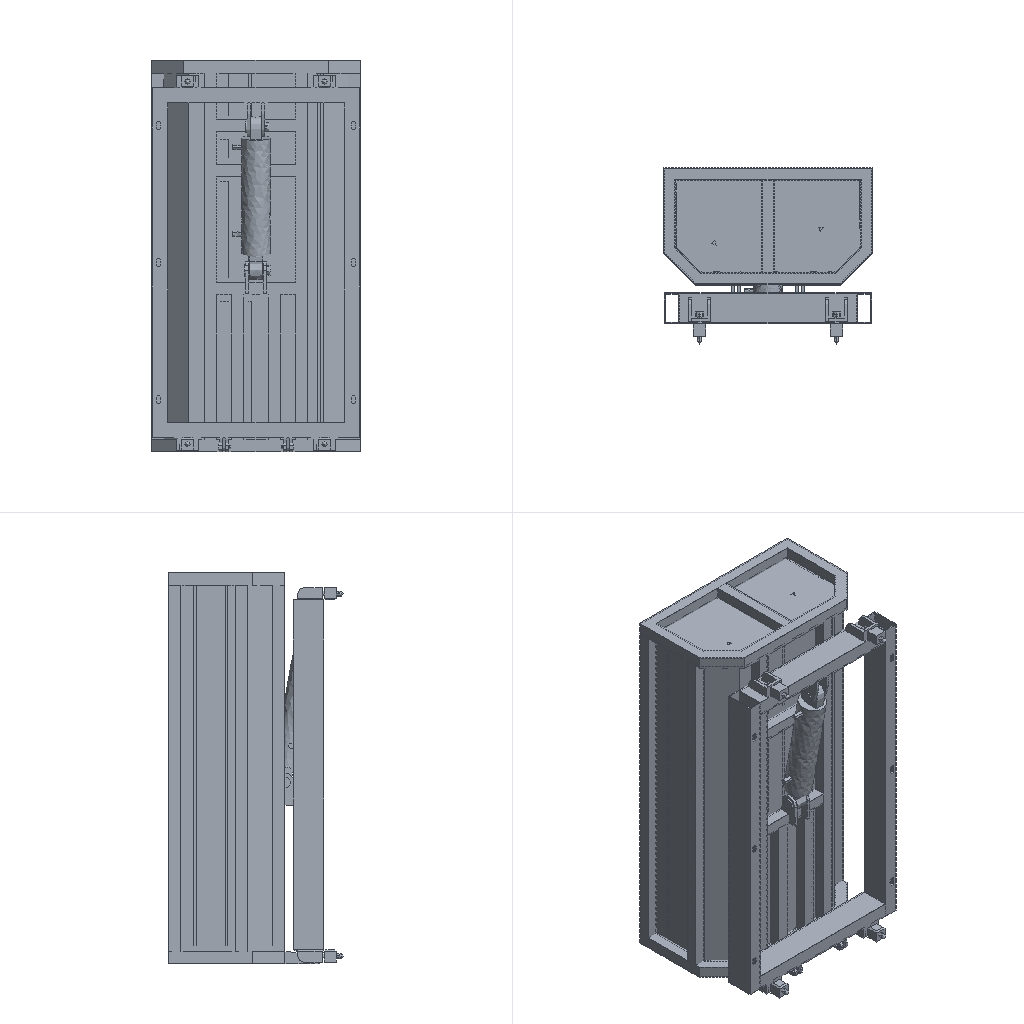Simulation study | ansys workbench
Ansys APDL input file, long lists of numbers shortened:
/batch
/config,noeldb,1     ! force off writing results to database
*get,_wallstrt,active,,time,wall
! ANSYS input file written by Workbench version 2022 R1
! File used for geometry attach:
/title,wbnew--____ (A5)
! ****** Begin Custom Load Command Snippet ******
/COM, ACT Extensions:
/COM,     LSDYNA, 2021.1
/COM,
! ****** End   Custom Load Command Snippet ******
*DIM,_wb_ProjectScratch_dir,string,248
_wb_ProjectScratch_dir(1) = ''
*DIM,_wb_SolverFiles_dir,string,248
_wb_SolverFiles_dir(1) = ''
*DIM,_wb_userfiles_dir,string,248
_wb_userfiles_dir(1) = ''
/com,--- Data in consistent MKS units. See Solving Units in the help system for more information.
/units,MKS
/nopr
/wb,file,start              !  signify a WB generated input file
/prep7
! Turn off shape checking because checks already performed inside WB mesher.
! See help system for more information.
SHPP,OFF,,NOWARN
/nolist
etcon,set             ! allow ANSYS to choose best KEYOP's for 180x elements, resets any applicable keyopt to MAPDL defaults
/com,*********** Nodes for the whole assembly ***********
nblock,3,,236970
(1i9,3e20.9e3)
        1    -3.888006712E-01    -1.500000000E-02    -1.150000000E+00
! (215427 more lines like these left out)
-1
/wb,elem,start            !  set before creation of elements
/com,*********** Elements for Body 1 "__\____-____1" ***********
et,1,186
keyo,1,2,1          ! set full integration on SOLID186
eblock,19,solid,,8694
(19i9)
        1        1        1        1        0        0        0        0       20        0     8776    28866    28867    30619    30620    30469    30468    32181    32180
! (17387 more lines like these left out)
-1
/com,*********** Elements for Body 2 "______3c_____3e_\__________________gb_Mt6728-2002 40__3(1)[1]" ***********
et,2,187
eblock,19,solid,,16742
(19i9)
        2        2        2        2        0        0        0        0       10        0    26722    98215   100703   101303   101302   114147   127238   114152   114151
! (33483 more lines like these left out)
-1
/com,*********** Elements for Body 3 "40X3_______3c_____3e_\____4[1]" ***********
et,3,187
eblock,19,solid,,5167
(19i9)
        3        3        3        3        0        0        0        0       10        0     3609    12186    13249    12762    12380    16239    19847    16237    16235
! (10333 more lines like these left out)
-1
/com,*********** Elements for Body 4 "40X3X1420____3c_____3e_\__________________(gb t6728-2002) 40__3(1)" ***********
et,4,186
keyo,4,2,1          ! set full integration on SOLID186
eblock,19,solid,,976
(19i9)
        4        4        4        4        0        0        0        0       20        0    68502   181284   182140   182324   181348   181346   182322   182323   181347
! (1951 more lines like these left out)
-1
/com,*********** Elements for Body 5 "40X3X1420____3c_____3e_\__________________(gb t6728-2002) 40__3(1)" ***********
et,5,186
keyo,5,2,1          ! set full integration on SOLID186
eblock,19,solid,,976
(19i9)
        5        5        5        5        0        0        0        0       20        0    69478   188196   189052   189236   188260   188258   189234   189235   188259
! (1951 more lines like these left out)
-1
! (41 more sections like these left out)
/wb,elem,end               !  done creating elements
/com,*********** Send User Defined Coordinate System(s) ***********
csys,0
toffst,273.15,  ! Temperature offset from absolute zero
/com,*********** Set Reference Temperature ***********
tref,22.
/wb,mat,start              !  starting to send materials
/com,*********** Send Materials ***********
Temperature = 'TEMP' ! Temperature
MP,DENS,1,7850,	! kg m^-3
MP,ALPX,1,1.2e-05,	! C^-1
MP,C,1,434,	! J kg^-1 C^-1
MP,KXX,1,60.5,	! W m^-1 C^-1
MP,RSVX,1,1.7e-07,	! kg m^3 A^-2 s^-3
MP,EX,1,200000000000,	! Pa
MP,NUXY,1,0.3,
MP,MURX,1,10000,
Temperature = 'TEMP' ! Temperature
MP,DENS,2,7850,	! kg m^-3
MP,ALPX,2,1.2e-05,	! C^-1
MP,C,2,434,	! J kg^-1 C^-1
MP,KXX,2,60.5,	! W m^-1 C^-1
MP,RSVX,2,1.7e-07,	! kg m^3 A^-2 s^-3
MP,EX,2,200000000000,	! Pa
MP,NUXY,2,0.3,
MP,MURX,2,10000,
Temperature = 'TEMP' ! Temperature
MP,DENS,3,7850,	! kg m^-3
MP,ALPX,3,1.2e-05,	! C^-1
MP,C,3,434,	! J kg^-1 C^-1
MP,KXX,3,60.5,	! W m^-1 C^-1
MP,RSVX,3,1.7e-07,	! kg m^3 A^-2 s^-3
MP,EX,3,200000000000,	! Pa
MP,NUXY,3,0.3,
MP,MURX,3,10000,
Temperature = 'TEMP' ! Temperature
MP,DENS,4,7850,	! kg m^-3
MP,ALPX,4,1.2e-05,	! C^-1
MP,C,4,434,	! J kg^-1 C^-1
MP,KXX,4,60.5,	! W m^-1 C^-1
MP,RSVX,4,1.7e-07,	! kg m^3 A^-2 s^-3
MP,EX,4,200000000000,	! Pa
MP,NUXY,4,0.3,
MP,MURX,4,10000,
Temperature = 'TEMP' ! Temperature
MP,DENS,5,7850,	! kg m^-3
MP,ALPX,5,1.2e-05,	! C^-1
MP,C,5,434,	! J kg^-1 C^-1
MP,KXX,5,60.5,	! W m^-1 C^-1
MP,RSVX,5,1.7e-07,	! kg m^3 A^-2 s^-3
MP,EX,5,200000000000,	! Pa
MP,NUXY,5,0.3,
MP,MURX,5,10000,
Temperature = 'TEMP' ! Temperature
MP,DENS,6,7850,	! kg m^-3
MP,ALPX,6,1.2e-05,	! C^-1
MP,C,6,434,	! J kg^-1 C^-1
MP,KXX,6,60.5,	! W m^-1 C^-1
MP,RSVX,6,1.7e-07,	! kg m^3 A^-2 s^-3
MP,EX,6,200000000000,	! Pa
MP,NUXY,6,0.3,
MP,MURX,6,10000,
Temperature = 'TEMP' ! Temperature
MP,DENS,7,7850,	! kg m^-3
MP,ALPX,7,1.2e-05,	! C^-1
MP,C,7,434,	! J kg^-1 C^-1
MP,KXX,7,60.5,	! W m^-1 C^-1
MP,RSVX,7,1.7e-07,	! kg m^3 A^-2 s^-3
MP,EX,7,200000000000,	! Pa
MP,NUXY,7,0.3,
MP,MURX,7,10000,
Temperature = 'TEMP' ! Temperature
MP,DENS,8,7850,	! kg m^-3
MP,ALPX,8,1.2e-05,	! C^-1
MP,C,8,434,	! J kg^-1 C^-1
MP,KXX,8,60.5,	! W m^-1 C^-1
MP,RSVX,8,1.7e-07,	! kg m^3 A^-2 s^-3
MP,EX,8,200000000000,	! Pa
MP,NUXY,8,0.3,
MP,MURX,8,10000,
Temperature = 'TEMP' ! Temperature
MP,DENS,9,7850,	! kg m^-3
MP,ALPX,9,1.2e-05,	! C^-1
MP,C,9,434,	! J kg^-1 C^-1
MP,KXX,9,60.5,	! W m^-1 C^-1
MP,RSVX,9,1.7e-07,	! kg m^3 A^-2 s^-3
MP,EX,9,200000000000,	! Pa
! (335 more lines like these left out)
/wb,mat,end                !  done sending materials
!************************* Model Summary ********************
!__\____-____1,	结构钢,	matid,	1
!______3c_____3e_\__________________gb_Mt6728-2002 40__3(1)[1],	结构钢,	matid,	2
!40X3_______3c_____3e_\____4[1],	结构钢,	matid,	3
! (45 more lines like these left out)
*get,_xmin,node,,mnloc,x
*get,_ymin,node,,mnloc,y
*get,_zmin,node,,mnloc,z
*get,_xmax,node,,mxloc,x
*get,_ymax,node,,mxloc,y
*get,_zmax,node,,mxloc,z
_ASMDIAG=(_xmax-_xmin)*(_xmax-_xmin)+(_ymax-_ymin)*(_ymax-_ymin)+(_zmax-_zmin)*(_zmax-_zmin)
_ASMDIAG=SQRT(_ASMDIAG)
/wb,contact,start          !  starting to send contact
/com,*********** Create Contact "接触区域" ***********
/com,            Real Constant Set For Above Contact Is 48 & 47
*set,tid,48
*set,cid,47
r,tid
r,cid
et,tid,170
et,cid,174
eblock,10,,,1504
(15i9)
   142848       48       48       48        0    25380    25381    25319    25318    47320    47139    47134    47135
! (1503 more lines like these left out)
-1
eblock,10,,,1504
(15i9)
   144352       47       47       47        0    25380    25381    25319    25318    47320    47139    47134    47135
! (1503 more lines like these left out)
-1
eblock,10,,,1368
(15i9)
   145856       47       48       47        0    97493   100730    99290    99290   108211   120892    99290   108208
! (1367 more lines like these left out)
-1
eblock,10,,,1368
(15i9)
   147224       48       47       48        0    97493   100730    99290    99290   108211   120892    99290   108208
! (1367 more lines like these left out)
-1
keyo,cid,8,2               ! auto create asymmetric contact (from Program Controlled setting)
keyo,cid,10,0              ! adjust contact stiffness each NR iteration (from Program Controlled setting)
keyo,cid,12,5              ! bonded always
keyo,cid,2,2               ! MPC contact.  Valid only for bonded or no separation.  Requires nodal detection
keyo,cid,4,2               ! on nodal point - normal to target surface (from Program Controlled setting)
keyo,cid,9,1               ! ignore initial gaps/penetration
keyo,cid,7,0               ! No Prediction
rmod,tid,3,10.      ! FKN
rmod,tid,5,0.       ! ICONT
rmod,tid,6,0.       ! PINB
rmod,tid,10,0.      ! CNOF
rmod,tid,12,0.      ! FKT
rmod,tid,36,161     ! WB DSID
rmod,cid,3,10.      ! FKN
rmod,cid,5,0.       ! ICONT
rmod,cid,6,0.       ! PINB
rmod,cid,10,0.      ! CNOF
rmod,cid,12,0.      ! FKT
rmod,cid,36,161     ! WB DSID
/com,*********** Create Contact "接触区域 2" ***********
/com,            Real Constant Set For Above Contact Is 50 & 49
*set,tid,50
*set,cid,49
r,tid
r,cid
et,tid,170
et,cid,174
eblock,10,,,378
(15i9)
   148592       50       50       50        0    24286    22612    22550    22549    39058    38934    38931    38932
! (377 more lines like these left out)
-1
eblock,10,,,378
(15i9)
   148970       49       49       49        0    24286    22612    22550    22549    39058    38934    38931    38932
! (377 more lines like these left out)
-1
eblock,10,,,440
(15i9)
   149348       49       50       49        0    12046    12616    13485    13485    15139    19132    13485    15144
! (439 more lines like these left out)
-1
eblock,10,,,440
(15i9)
   149788       50       49       50        0    12046    12616    13485    13485    15139    19132    13485    15144
! (439 more lines like these left out)
-1
keyo,cid,8,2               ! auto create asymmetric contact (from Program Controlled setting)
keyo,cid,10,0              ! adjust contact stiffness each NR iteration (from Program Controlled setting)
keyo,cid,12,5              ! bonded always
keyo,cid,2,2               ! MPC contact.  Valid only for bonded or no separation.  Requires nodal detection
keyo,cid,4,2               ! on nodal point - normal to target surface (from Program Controlled setting)
keyo,cid,9,1               ! ignore initial gaps/penetration
keyo,cid,7,0               ! No Prediction
rmod,tid,3,10.      ! FKN
rmod,tid,5,0.       ! ICONT
rmod,tid,6,0.       ! PINB
rmod,tid,10,0.      ! CNOF
rmod,tid,12,0.      ! FKT
rmod,tid,36,164     ! WB DSID
rmod,cid,3,10.      ! FKN
rmod,cid,5,0.       ! ICONT
rmod,cid,6,0.       ! PINB
rmod,cid,10,0.      ! CNOF
rmod,cid,12,0.      ! FKT
rmod,cid,36,164     ! WB DSID
/com,*********** Create Contact "接触区域 3" ***********
/com,            Real Constant Set For Above Contact Is 52 & 51
*set,tid,52
*set,cid,51
r,tid
r,cid
et,tid,170
et,cid,174
eblock,10,,,372
(15i9)
   150228       52       52       52        0    22612    22613    22551    22550    39056    38936    38933    38934
! (371 more lines like these left out)
-1
eblock,10,,,372
(15i9)
   150600       51       51       51        0    22612    22613    22551    22550    39056    38936    38933    38934
! (371 more lines like these left out)
-1
eblock,10,,,244
(15i9)
   150972       51       52       51        0   181588   181408   181348   181347   185076   184896   184892   184893
! (243 more lines like these left out)
-1
eblock,10,,,244
(15i9)
   151216       52       51       52        0   181588   181408   181348   181347   185076   184896   184892   184893
! (243 more lines like these left out)
-1
keyo,cid,8,2               ! auto create asymmetric contact (from Program Controlled setting)
keyo,cid,10,0              ! adjust contact stiffness each NR iteration (from Program Controlled setting)
keyo,cid,12,5              ! bonded always
keyo,cid,2,2               ! MPC contact.  Valid only for bonded or no separation.  Requires nodal detection
keyo,cid,4,2               ! on nodal point - normal to target surface (from Program Controlled setting)
keyo,cid,9,1               ! ignore initial gaps/penetration
keyo,cid,7,0               ! No Prediction
rmod,tid,3,10.      ! FKN
rmod,tid,5,0.       ! ICONT
rmod,tid,6,0.       ! PINB
rmod,tid,10,0.      ! CNOF
rmod,tid,12,0.      ! FKT
rmod,tid,36,167     ! WB DSID
rmod,cid,3,10.      ! FKN
rmod,cid,5,0.       ! ICONT
rmod,cid,6,0.       ! PINB
rmod,cid,10,0.      ! CNOF
rmod,cid,12,0.      ! FKT
rmod,cid,36,167     ! WB DSID
/com,*********** Create Contact "接触区域 4" ***********
/com,            Real Constant Set For Above Contact Is 54 & 53
*set,tid,54
*set,cid,53
r,tid
r,cid
et,tid,170
et,cid,174
eblock,10,,,310
(15i9)
   151460       54       54       54        0    30489    28875    28849    30488    58530    58425    58427    63314
! (309 more lines like these left out)
-1
eblock,10,,,310
(15i9)
   151770       53       53       53        0    30489    28875    28849    30488    58530    58425    58427    63314
! (309 more lines like these left out)
-1
eblock,10,,,244
(15i9)
   152080       53       54       53        0   188012   187832   187772   187771   190532   190352   190348   190349
! (243 more lines like these left out)
-1
eblock,10,,,244
(15i9)
   152324       54       53       54        0   188012   187832   187772   187771   190532   190352   190348   190349
! (243 more lines like these left out)
-1
keyo,cid,8,2               ! auto create asymmetric contact (from Program Controlled setting)
keyo,cid,10,0              ! adjust contact stiffness each NR iteration (from Program Controlled setting)
keyo,cid,12,5              ! bonded always
keyo,cid,2,2               ! MPC contact.  Valid only for bonded or no separation.  Requires nodal detection
keyo,cid,4,2               ! on nodal point - normal to target surface (from Program Controlled setting)
keyo,cid,9,1               ! ignore initial gaps/penetration
keyo,cid,7,0               ! No Prediction
rmod,tid,3,10.      ! FKN
rmod,tid,5,0.       ! ICONT
rmod,tid,6,0.       ! PINB
rmod,tid,10,0.      ! CNOF
rmod,tid,12,0.      ! FKT
rmod,tid,36,170     ! WB DSID
rmod,cid,3,10.      ! FKN
rmod,cid,5,0.       ! ICONT
rmod,cid,6,0.       ! PINB
rmod,cid,10,0.      ! CNOF
rmod,cid,12,0.      ! FKT
rmod,cid,36,170     ! WB DSID
/com,*********** Create Contact "接触区域 5" ***********
/com,            Real Constant Set For Above Contact Is 56 & 55
*set,tid,56
*set,cid,55
r,tid
r,cid
et,tid,170
et,cid,174
eblock,10,,,310
(15i9)
   152568       56       56       56        0    28896    28897    28871    28870    58592    58514    58509    58510
! (309 more lines like these left out)
-1
eblock,10,,,310
(15i9)
   152878       55       55       55        0    28896    28897    28871    28870    58592    58514    58509    58510
! (309 more lines like these left out)
-1
eblock,10,,,244
(15i9)
   153188       55       56       55        0   194924   194744   194684   194683   197444   197264   197260   197261
! (243 more lines like these left out)
-1
eblock,10,,,244
(15i9)
   153432       56       55       56        0   194924   194744   194684   194683   197444   197264   197260   197261
! (243 more lines like these left out)
-1
keyo,cid,8,2               ! auto create asymmetric contact (from Program Controlled setting)
keyo,cid,10,0              ! adjust contact stiffness each NR iteration (from Program Controlled setting)
keyo,cid,12,5              ! bonded always
keyo,cid,2,2               ! MPC contact.  Valid only for bonded or no separation.  Requires nodal detection
keyo,cid,4,2               ! on nodal point - normal to target surface (from Program Controlled setting)
keyo,cid,9,1               ! ignore initial gaps/penetration
keyo,cid,7,0               ! No Prediction
rmod,tid,3,10.      ! FKN
rmod,tid,5,0.       ! ICONT
rmod,tid,6,0.       ! PINB
rmod,tid,10,0.      ! CNOF
rmod,tid,12,0.      ! FKT
rmod,tid,36,173     ! WB DSID
rmod,cid,3,10.      ! FKN
rmod,cid,5,0.       ! ICONT
rmod,cid,6,0.       ! PINB
rmod,cid,10,0.      ! CNOF
rmod,cid,12,0.      ! FKT
rmod,cid,36,173     ! WB DSID
! (70 more sections like these left out)
/wb,contact,end            !  done creating contacts
/golist
/wb,load,start             !  starting to send loads
/com,*********** Fixed Supports ***********
CMBLOCK,_FIXEDSU,NODE,       84
(8i10)
    208263    208264    208265    208266    208267    208268    208269    208270
! (10 more lines like these left out)
cmsel,s,_FIXEDSU
d,all,all
nsel,all
/com,*********** Define Force Using Surface Effect Elements ***********
local,12,0,0.,0.,0.,0.,0.,0.
csys,0
et,197,154
eblock,10,,,678
(15i9)
   164632      197      197      197       12     7376     7377     6933     6933    10000     8678     6933     8677
! (677 more lines like these left out)
-1
esel,s,type,,197
keyop,197,2,1                ! Apply load in local coordinate system
keyop,197,7,1                ! Use original area so load is constant in large deformation
esel,all
/gst,on,on
fini
*get,_numnode,node,0,count
*get,_numelem,elem,0,count
*get, _MAXELEMNUM, elem, 0, NUM, MAX
*get, _MAXNODENUM, node, 0, NUM, MAX
*get, _MAXELEMTYPE, etyp, 0, NUM, MAX
*get, _MAXREALCONST, real, 0, NUM, MAX
/go
/wb,load,end               !  done creating loads
/com,--- Number of total nodes = %_numnode%
/com,--- Number of contact elements = 22462
/com,--- Number of spring elements = 0
/com,--- Number of bearing elements = 0
/com,--- Number of solid elements = 75325
/com,--- Number of condensed parts = 0
/com,--- Number of total elements = %_numelem%
*get,_wallbsol,active,,time,wall
/com,****************************************************************************
/com,*************************    SOLUTION       ********************************
/com,****************************************************************************
/solu
antype,0                   ! static analysis
neqit,1,force              ! Force 1 eq iteration since only nonlinearity is bonded/no sep contact
pred,off
_thickRatio=0.0435  ! Ratio of thick parts in the model
eqsl,sparse,,,,,1
cntr,print,1               ! print out contact info and also make no initial contact an error
dmpoption,emat,no             ! Don't combine emat file for DANSYS
dmpoption,esav,no             ! Don't combine esav file for DANSYS
nldiag,cont,iter           ! print out contact info each equilibrium iteration
rescontrol,,none                 ! Do not keep any restart files
/com,****************************************************
/com,******************* SOLVE FOR LS 1 OF 1 ****************
esel,s,type,,197
nsle
sfe,all,1,pres,1,0.
sfe,all,2,pres,1,0.
sfe,all,3,pres,1,5960.108
nsel,all
esel,all
/nopr
/gopr
nsub,1,1,1
time,1.
outres,erase
outres,all,none
outres,nsol,all,
outres,rsol,all
outres,eangl,all
outres,etmp,all
outres,veng,all
outres,strs,all,
outres,epel,all,
outres,eppl,all,
outres,cont,all,
! *********** WB SOLVE COMMAND ***********
! check interactive state
*get,ANSINTER_,active,,int
*if,ANSINTER_,ne,0,then
/eof
*endif
solve
/com *************** Write FE CONNECTORS *********
CEWRITE,file,ce,,INTE
/com,****************************************************
/com,*************** FINISHED SOLVE FOR LS 1 *************
*get,_wallasol,active,,time,wall
/nopr
*get,_numnode,node,0,count
*get,_numelem,elem,0,count
*get, _MAXELEMNUM, elem, 0, NUM, MAX
*get, _MAXNODENUM, node, 0, NUM, MAX,,,INTERNAL
*get, _MAXELEMTYPE, etyp, 0, NUM, MAX
*get, _MAXREALCONST, real, 0, NUM, MAX
/gopr
/post1
xmlo,ENCODING,ISO-8859-1
xmlo,parm
/xml,parm,xml
fini
/gopr
*get,_walldone,active,,time,wall
_preptime=(_wallbsol-_wallstrt)*3600
_solvtime=(_wallasol-_wallbsol)*3600
_posttime=(_walldone-_wallasol)*3600
_totaltim=(_walldone-_wallstrt)*3600
*get,_dlbratio,active,0,solu,dlbr
*get,_combtime,active,0,solu,comb
*get,_ssmode,active,0,solu,ssmm
*get,_ndofs,active,0,solu,ndof
*get,_sol_end_time,active,0,set,time
*if,_sol_end_time,eq,1.,then
/fclean				!clean distributed files
*endif
/com,--- Total number of nodes = %_numnode%
/com,--- Total number of elements = %_numelem%
/com,--- Element load balance ratio = %_dlbratio%
/com,--- Time to combine distributed files = %_combtime%
/com,--- Sparse memory mode = %_ssmode%
/com,--- Number of DOF = %_ndofs%
/wb,file,end               ! done with WB generated input